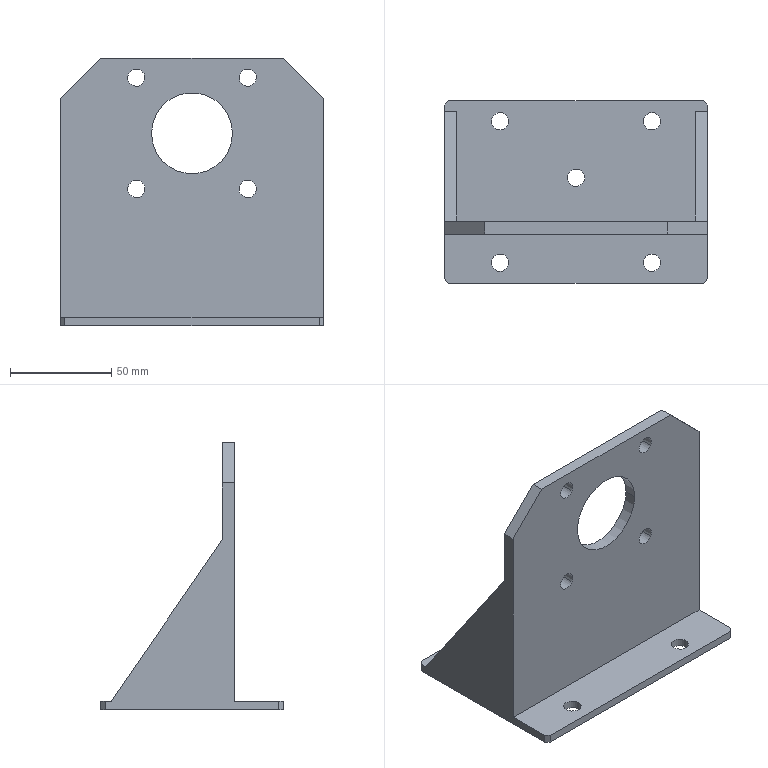Part | STEP file | 20314 | 1 solid | 40 faces | box 130 x 90 x 132 mm | volume 160571 mm3 | cylinder 20 | plane 20 | commonest cylinder face diameters 8.5 x18 40 x2
STEP:
#1=CARTESIAN_POINT('',(23.77,-15.,124.538));
#2=VERTEX_POINT('',#1);
#3=CARTESIAN_POINT('',(23.77,-21.,124.538));
#4=VERTEX_POINT('',#3);
#5=CARTESIAN_POINT('',(23.77,-28.155,124.538));
#6=DIRECTION('',(0.,1.,0.));
#7=VECTOR('',#6,1.);
#8=LINE('',#5,#7);
#9=EDGE_CURVE('',#2,#4,#8,.F.);
#10=ORIENTED_EDGE('',*,*,#9,.F.);
#11=CARTESIAN_POINT('',(31.23,-15.,120.462));
#12=VERTEX_POINT('',#11);
#13=CARTESIAN_POINT('',(27.5,-15.,122.5));
#14=DIRECTION('',(0.,1.,0.));
#15=AXIS2_PLACEMENT_3D('',#13,#14,$);
#16=CIRCLE('',#15,4.25);
#17=EDGE_CURVE('',#12,#2,#16,.F.);
#18=ORIENTED_EDGE('',*,*,#17,.F.);
#19=CARTESIAN_POINT('',(31.23,-21.,120.462));
#20=VERTEX_POINT('',#19);
#21=CARTESIAN_POINT('',(31.23,-28.155,120.462));
#22=DIRECTION('',(0.,1.,0.));
#23=VECTOR('',#22,1.);
#24=LINE('',#21,#23);
#25=EDGE_CURVE('',#12,#20,#24,.F.);
#26=ORIENTED_EDGE('',*,*,#25,.T.);
#27=CARTESIAN_POINT('',(27.5,-21.,122.5));
#28=DIRECTION('',(0.,1.,0.));
#29=AXIS2_PLACEMENT_3D('',#27,#28,$);
#30=CIRCLE('',#29,4.25);
#31=EDGE_CURVE('',#4,#20,#30,.T.);
#32=ORIENTED_EDGE('',*,*,#31,.F.);
#33=EDGE_LOOP('',(#10,#18,#26,#32));
#34=FACE_OUTER_BOUND('',#33,.T.);
#35=CARTESIAN_POINT('',(27.5,-20.9,122.5));
#36=DIRECTION('',(0.,1.,0.));
#37=DIRECTION('',(0.8776,0.,-0.4794));
#38=AXIS2_PLACEMENT_3D('',#35,#36,#37);
#39=CYLINDRICAL_SURFACE('',#38,4.25);
#40=ADVANCED_FACE('',(#34),#39,.F.);
#41=ORIENTED_EDGE('',*,*,#25,.F.);
#42=CARTESIAN_POINT('',(27.5,-15.,122.5));
#43=DIRECTION('',(0.,1.,0.));
#44=AXIS2_PLACEMENT_3D('',#42,#43,$);
#45=CIRCLE('',#44,4.25);
#46=EDGE_CURVE('',#2,#12,#45,.F.);
#47=ORIENTED_EDGE('',*,*,#46,.F.);
#48=ORIENTED_EDGE('',*,*,#9,.T.);
#49=CARTESIAN_POINT('',(27.5,-21.,122.5));
#50=DIRECTION('',(0.,1.,0.));
#51=AXIS2_PLACEMENT_3D('',#49,#50,$);
#52=CIRCLE('',#51,4.25);
#53=EDGE_CURVE('',#20,#4,#52,.T.);
#54=ORIENTED_EDGE('',*,*,#53,.F.);
#55=EDGE_LOOP('',(#41,#47,#48,#54));
#56=FACE_OUTER_BOUND('',#55,.T.);
#57=ADVANCED_FACE('',(#56),#39,.F.);
#58=CARTESIAN_POINT('',(65.,-21.,112.));
#59=VERTEX_POINT('',#58);
#60=CARTESIAN_POINT('',(65.,-15.,112.));
#61=VERTEX_POINT('',#60);
#62=CARTESIAN_POINT('',(65.,-18.,112.));
#63=DIRECTION('',(0.,1.,0.));
#64=VECTOR('',#63,1.);
#65=LINE('',#62,#64);
#66=EDGE_CURVE('',#59,#61,#65,.T.);
#67=ORIENTED_EDGE('',*,*,#66,.F.);
#68=CARTESIAN_POINT('',(65.,-21.,4.));
#69=VERTEX_POINT('',#68);
#70=CARTESIAN_POINT('',(65.,-21.,58.));
#71=DIRECTION('',(0.,0.,1.));
#72=VECTOR('',#71,1.);
#73=LINE('',#70,#72);
#74=EDGE_CURVE('',#69,#59,#73,.T.);
#75=ORIENTED_EDGE('',*,*,#74,.F.);
#76=CARTESIAN_POINT('',(65.,-43.,4.));
#77=VERTEX_POINT('',#76);
#78=CARTESIAN_POINT('',(65.,-32.,4.));
#79=DIRECTION('',(0.,-1.,0.));
#80=VECTOR('',#79,1.);
#81=LINE('',#78,#80);
#82=EDGE_CURVE('',#77,#69,#81,.F.);
#83=ORIENTED_EDGE('',*,*,#82,.F.);
#84=CARTESIAN_POINT('',(65.,-43.,0.));
#85=VERTEX_POINT('',#84);
#86=CARTESIAN_POINT('',(65.,-43.,2.));
#87=DIRECTION('',(0.,0.,1.));
#88=VECTOR('',#87,1.);
#89=LINE('',#86,#88);
#90=EDGE_CURVE('',#85,#77,#89,.T.);
#91=ORIENTED_EDGE('',*,*,#90,.F.);
#92=CARTESIAN_POINT('',(65.,43.,0.));
#93=VERTEX_POINT('',#92);
#94=CARTESIAN_POINT('',(65.,0.,0.));
#95=DIRECTION('',(0.,-1.,0.));
#96=VECTOR('',#95,1.);
#97=LINE('',#94,#96);
#98=EDGE_CURVE('',#85,#93,#97,.F.);
#99=ORIENTED_EDGE('',*,*,#98,.T.);
#100=CARTESIAN_POINT('',(65.,43.,4.));
#101=VERTEX_POINT('',#100);
#102=CARTESIAN_POINT('',(65.,43.,2.));
#103=DIRECTION('',(0.,0.,-1.));
#104=VECTOR('',#103,1.);
#105=LINE('',#102,#104);
#106=EDGE_CURVE('',#93,#101,#105,.F.);
#107=ORIENTED_EDGE('',*,*,#106,.T.);
#108=CARTESIAN_POINT('',(65.,40.,4.));
#109=VERTEX_POINT('',#108);
#110=CARTESIAN_POINT('',(65.,41.5,4.));
#111=DIRECTION('',(0.,-1.,0.));
#112=VECTOR('',#111,1.);
#113=LINE('',#110,#112);
#114=EDGE_CURVE('',#109,#101,#113,.F.);
#115=ORIENTED_EDGE('',*,*,#114,.F.);
#116=CARTESIAN_POINT('',(65.,-15.,84.));
#117=VERTEX_POINT('',#116);
#118=CARTESIAN_POINT('',(65.,12.5,44.));
#119=DIRECTION('',(0.,0.5665,-0.824));
#120=VECTOR('',#119,1.);
#121=LINE('',#118,#120);
#122=EDGE_CURVE('',#117,#109,#121,.T.);
#123=ORIENTED_EDGE('',*,*,#122,.F.);
#124=CARTESIAN_POINT('',(65.,-15.,98.));
#125=DIRECTION('',(0.,0.,1.));
#126=VECTOR('',#125,1.);
#127=LINE('',#124,#126);
#128=EDGE_CURVE('',#117,#61,#127,.T.);
#129=ORIENTED_EDGE('',*,*,#128,.T.);
#130=EDGE_LOOP('',(#67,#75,#83,#91,#99,#107,#115,#123,#129));
#131=FACE_OUTER_BOUND('',#130,.T.);
#132=CARTESIAN_POINT('',(65.,45.,0.));
#133=DIRECTION('',(-1.,0.,0.));
#134=DIRECTION('',(0.,-1.,0.));
#135=AXIS2_PLACEMENT_3D('',#132,#133,#134);
#136=PLANE('',#135);
#137=ADVANCED_FACE('',(#131),#136,.F.);
#138=CARTESIAN_POINT('',(-65.,-21.,4.));
#139=VERTEX_POINT('',#138);
#140=CARTESIAN_POINT('',(-65.,-43.,4.));
#141=VERTEX_POINT('',#140);
#142=CARTESIAN_POINT('',(-65.,-32.,4.));
#143=DIRECTION('',(0.,1.,0.));
#144=VECTOR('',#143,1.);
#145=LINE('',#142,#144);
#146=EDGE_CURVE('',#139,#141,#145,.F.);
#147=ORIENTED_EDGE('',*,*,#146,.T.);
#148=CARTESIAN_POINT('',(-63.,-45.,4.));
#149=VERTEX_POINT('',#148);
#150=CARTESIAN_POINT('',(-64.,-44.,4.));
#151=DIRECTION('',(0.7071,-0.7071,0.));
#152=VECTOR('',#151,1.);
#153=LINE('',#150,#152);
#154=EDGE_CURVE('',#149,#141,#153,.F.);
#155=ORIENTED_EDGE('',*,*,#154,.F.);
#156=CARTESIAN_POINT('',(63.,-45.,4.));
#157=VERTEX_POINT('',#156);
#158=CARTESIAN_POINT('',(0.,-45.,4.));
#159=DIRECTION('',(-1.,0.,0.));
#160=VECTOR('',#159,1.);
#161=LINE('',#158,#160);
#162=EDGE_CURVE('',#149,#157,#161,.F.);
#163=ORIENTED_EDGE('',*,*,#162,.T.);
#164=CARTESIAN_POINT('',(64.,-44.,4.));
#165=DIRECTION('',(-0.7071,-0.7071,0.));
#166=VECTOR('',#165,1.);
#167=LINE('',#164,#166);
#168=EDGE_CURVE('',#77,#157,#167,.T.);
#169=ORIENTED_EDGE('',*,*,#168,.F.);
#170=ORIENTED_EDGE('',*,*,#82,.T.);
#171=CARTESIAN_POINT('',(0.,-21.,4.));
#172=DIRECTION('',(-1.,0.,0.));
#173=VECTOR('',#172,1.);
#174=LINE('',#171,#173);
#175=EDGE_CURVE('',#139,#69,#174,.F.);
#176=ORIENTED_EDGE('',*,*,#175,.F.);
#177=EDGE_LOOP('',(#147,#155,#163,#169,#170,#176));
#178=FACE_OUTER_BOUND('',#177,.T.);
#179=CARTESIAN_POINT('',(41.23,-37.038,4.));
#180=VERTEX_POINT('',#179);
#181=CARTESIAN_POINT('',(33.77,-32.962,4.));
#182=VERTEX_POINT('',#181);
#183=CARTESIAN_POINT('',(37.5,-35.,4.));
#184=DIRECTION('',(0.,0.,1.));
#185=AXIS2_PLACEMENT_3D('',#183,#184,$);
#186=CIRCLE('',#185,4.25);
#187=EDGE_CURVE('',#180,#182,#186,.T.);
#188=ORIENTED_EDGE('',*,*,#187,.F.);
#189=CARTESIAN_POINT('',(37.5,-35.,4.));
#190=DIRECTION('',(0.,0.,1.));
#191=AXIS2_PLACEMENT_3D('',#189,#190,$);
#192=CIRCLE('',#191,4.25);
#193=EDGE_CURVE('',#182,#180,#192,.T.);
#194=ORIENTED_EDGE('',*,*,#193,.F.);
#195=EDGE_LOOP('',(#188,#194));
#196=FACE_BOUND('',#195,.T.);
#197=CARTESIAN_POINT('',(-33.77,-37.038,4.));
#198=VERTEX_POINT('',#197);
#199=CARTESIAN_POINT('',(-41.23,-32.962,4.));
#200=VERTEX_POINT('',#199);
#201=CARTESIAN_POINT('',(-37.5,-35.,4.));
#202=DIRECTION('',(0.,0.,1.));
#203=AXIS2_PLACEMENT_3D('',#201,#202,$);
#204=CIRCLE('',#203,4.25);
#205=EDGE_CURVE('',#198,#200,#204,.T.);
#206=ORIENTED_EDGE('',*,*,#205,.F.);
#207=CARTESIAN_POINT('',(-37.5,-35.,4.));
#208=DIRECTION('',(0.,0.,1.));
#209=AXIS2_PLACEMENT_3D('',#207,#208,$);
#210=CIRCLE('',#209,4.25);
#211=EDGE_CURVE('',#200,#198,#210,.T.);
#212=ORIENTED_EDGE('',*,*,#211,.F.);
#213=EDGE_LOOP('',(#206,#212));
#214=FACE_BOUND('',#213,.T.);
#215=CARTESIAN_POINT('',(0.,0.,4.));
#216=DIRECTION('',(0.,0.,1.));
#217=DIRECTION('',(1.,0.,0.));
#218=AXIS2_PLACEMENT_3D('',#215,#216,#217);
#219=PLANE('',#218);
#220=ADVANCED_FACE('',(#178,#196,#214),#219,.T.);
#221=ORIENTED_EDGE('',*,*,#106,.F.);
#222=CARTESIAN_POINT('',(63.,45.,0.));
#223=VERTEX_POINT('',#222);
#224=CARTESIAN_POINT('',(64.,44.,0.));
#225=DIRECTION('',(0.7071,-0.7071,0.));
#226=VECTOR('',#225,1.);
#227=LINE('',#224,#226);
#228=EDGE_CURVE('',#93,#223,#227,.F.);
#229=ORIENTED_EDGE('',*,*,#228,.T.);
#230=CARTESIAN_POINT('',(63.,45.,4.));
#231=VERTEX_POINT('',#230);
#232=CARTESIAN_POINT('',(63.,45.,2.));
#233=DIRECTION('',(0.,0.,-1.));
#234=VECTOR('',#233,1.);
#235=LINE('',#232,#234);
#236=EDGE_CURVE('',#223,#231,#235,.F.);
#237=ORIENTED_EDGE('',*,*,#236,.T.);
#238=CARTESIAN_POINT('',(64.,44.,4.));
#239=DIRECTION('',(0.7071,-0.7071,0.));
#240=VECTOR('',#239,1.);
#241=LINE('',#238,#240);
#242=EDGE_CURVE('',#231,#101,#241,.T.);
#243=ORIENTED_EDGE('',*,*,#242,.T.);
#244=EDGE_LOOP('',(#221,#229,#237,#243));
#245=FACE_OUTER_BOUND('',#244,.T.);
#246=CARTESIAN_POINT('',(63.,45.,4.8));
#247=DIRECTION('',(-0.7071,-0.7071,0.));
#248=DIRECTION('',(0.,0.,-1.));
#249=AXIS2_PLACEMENT_3D('',#246,#247,#248);
#250=PLANE('',#249);
#251=ADVANCED_FACE('',(#245),#250,.F.);
#252=CARTESIAN_POINT('',(-65.,-43.,0.));
#253=VERTEX_POINT('',#252);
#254=CARTESIAN_POINT('',(-63.,-45.,0.));
#255=VERTEX_POINT('',#254);
#256=CARTESIAN_POINT('',(-64.,-44.,0.));
#257=DIRECTION('',(0.7071,-0.7071,0.));
#258=VECTOR('',#257,1.);
#259=LINE('',#256,#258);
#260=EDGE_CURVE('',#253,#255,#259,.T.);
#261=ORIENTED_EDGE('',*,*,#260,.F.);
#262=CARTESIAN_POINT('',(-65.,43.,0.));
#263=VERTEX_POINT('',#262);
#264=CARTESIAN_POINT('',(-65.,0.,0.));
#265=DIRECTION('',(0.,1.,0.));
#266=VECTOR('',#265,1.);
#267=LINE('',#264,#266);
#268=EDGE_CURVE('',#263,#253,#267,.F.);
#269=ORIENTED_EDGE('',*,*,#268,.F.);
#270=CARTESIAN_POINT('',(-63.,45.,0.));
#271=VERTEX_POINT('',#270);
#272=CARTESIAN_POINT('',(-64.,44.,0.));
#273=DIRECTION('',(0.7071,0.7071,0.));
#274=VECTOR('',#273,1.);
#275=LINE('',#272,#274);
#276=EDGE_CURVE('',#271,#263,#275,.F.);
#277=ORIENTED_EDGE('',*,*,#276,.F.);
#278=CARTESIAN_POINT('',(0.,45.,0.));
#279=DIRECTION('',(1.,0.,0.));
#280=VECTOR('',#279,1.);
#281=LINE('',#278,#280);
#282=EDGE_CURVE('',#223,#271,#281,.F.);
#283=ORIENTED_EDGE('',*,*,#282,.F.);
#284=ORIENTED_EDGE('',*,*,#228,.F.);
#285=ORIENTED_EDGE('',*,*,#98,.F.);
#286=CARTESIAN_POINT('',(63.,-45.,0.));
#287=VERTEX_POINT('',#286);
#288=CARTESIAN_POINT('',(64.,-44.,0.));
#289=DIRECTION('',(-0.7071,-0.7071,0.));
#290=VECTOR('',#289,1.);
#291=LINE('',#288,#290);
#292=EDGE_CURVE('',#287,#85,#291,.F.);
#293=ORIENTED_EDGE('',*,*,#292,.F.);
#294=CARTESIAN_POINT('',(0.,-45.,0.));
#295=DIRECTION('',(-1.,0.,0.));
#296=VECTOR('',#295,1.);
#297=LINE('',#294,#296);
#298=EDGE_CURVE('',#255,#287,#297,.F.);
#299=ORIENTED_EDGE('',*,*,#298,.F.);
#300=EDGE_LOOP('',(#261,#269,#277,#283,#284,#285,#293,#299));
#301=FACE_OUTER_BOUND('',#300,.T.);
#302=CARTESIAN_POINT('',(33.77,-32.962,0.));
#303=VERTEX_POINT('',#302);
#304=CARTESIAN_POINT('',(41.23,-37.038,0.));
#305=VERTEX_POINT('',#304);
#306=CARTESIAN_POINT('',(37.5,-35.,0.));
#307=DIRECTION('',(0.,0.,1.));
#308=AXIS2_PLACEMENT_3D('',#306,#307,$);
#309=CIRCLE('',#308,4.25);
#310=EDGE_CURVE('',#303,#305,#309,.T.);
#311=ORIENTED_EDGE('',*,*,#310,.T.);
#312=CARTESIAN_POINT('',(37.5,-35.,0.));
#313=DIRECTION('',(0.,0.,1.));
#314=AXIS2_PLACEMENT_3D('',#312,#313,$);
#315=CIRCLE('',#314,4.25);
#316=EDGE_CURVE('',#305,#303,#315,.T.);
#317=ORIENTED_EDGE('',*,*,#316,.T.);
#318=EDGE_LOOP('',(#311,#317));
#319=FACE_BOUND('',#318,.T.);
#320=CARTESIAN_POINT('',(41.23,32.962,0.));
#321=VERTEX_POINT('',#320);
#322=CARTESIAN_POINT('',(33.77,37.038,0.));
#323=VERTEX_POINT('',#322);
#324=CARTESIAN_POINT('',(37.5,35.,0.));
#325=DIRECTION('',(0.,0.,1.));
#326=AXIS2_PLACEMENT_3D('',#324,#325,$);
#327=CIRCLE('',#326,4.25);
#328=EDGE_CURVE('',#321,#323,#327,.T.);
#329=ORIENTED_EDGE('',*,*,#328,.T.);
#330=CARTESIAN_POINT('',(37.5,35.,0.));
#331=DIRECTION('',(0.,0.,1.));
#332=AXIS2_PLACEMENT_3D('',#330,#331,$);
#333=CIRCLE('',#332,4.25);
#334=EDGE_CURVE('',#323,#321,#333,.T.);
#335=ORIENTED_EDGE('',*,*,#334,.T.);
#336=EDGE_LOOP('',(#329,#335));
#337=FACE_BOUND('',#336,.T.);
#338=CARTESIAN_POINT('',(-41.23,-32.962,0.));
#339=VERTEX_POINT('',#338);
#340=CARTESIAN_POINT('',(-33.77,-37.038,0.));
#341=VERTEX_POINT('',#340);
#342=CARTESIAN_POINT('',(-37.5,-35.,0.));
#343=DIRECTION('',(0.,0.,1.));
#344=AXIS2_PLACEMENT_3D('',#342,#343,$);
#345=CIRCLE('',#344,4.25);
#346=EDGE_CURVE('',#339,#341,#345,.T.);
#347=ORIENTED_EDGE('',*,*,#346,.T.);
#348=CARTESIAN_POINT('',(-37.5,-35.,0.));
#349=DIRECTION('',(0.,0.,1.));
#350=AXIS2_PLACEMENT_3D('',#348,#349,$);
#351=CIRCLE('',#350,4.25);
#352=EDGE_CURVE('',#341,#339,#351,.T.);
#353=ORIENTED_EDGE('',*,*,#352,.T.);
#354=EDGE_LOOP('',(#347,#353));
#355=FACE_BOUND('',#354,.T.);
#356=CARTESIAN_POINT('',(-41.23,37.038,0.));
#357=VERTEX_POINT('',#356);
#358=CARTESIAN_POINT('',(-33.77,32.962,0.));
#359=VERTEX_POINT('',#358);
#360=CARTESIAN_POINT('',(-37.5,35.,0.));
#361=DIRECTION('',(0.,0.,1.));
#362=AXIS2_PLACEMENT_3D('',#360,#361,$);
#363=CIRCLE('',#362,4.25);
#364=EDGE_CURVE('',#357,#359,#363,.T.);
#365=ORIENTED_EDGE('',*,*,#364,.T.);
#366=CARTESIAN_POINT('',(-37.5,35.,0.));
#367=DIRECTION('',(0.,0.,1.));
#368=AXIS2_PLACEMENT_3D('',#366,#367,$);
#369=CIRCLE('',#368,4.25);
#370=EDGE_CURVE('',#359,#357,#369,.T.);
#371=ORIENTED_EDGE('',*,*,#370,.T.);
#372=EDGE_LOOP('',(#365,#371));
#373=FACE_BOUND('',#372,.T.);
#374=CARTESIAN_POINT('',(-3.73,9.038,0.));
#375=VERTEX_POINT('',#374);
#376=CARTESIAN_POINT('',(3.73,4.962,0.));
#377=VERTEX_POINT('',#376);
#378=CARTESIAN_POINT('',(0.,7.,0.));
#379=DIRECTION('',(0.,0.,1.));
#380=AXIS2_PLACEMENT_3D('',#378,#379,$);
#381=CIRCLE('',#380,4.25);
#382=EDGE_CURVE('',#375,#377,#381,.T.);
#383=ORIENTED_EDGE('',*,*,#382,.T.);
#384=CARTESIAN_POINT('',(0.,7.,0.));
#385=DIRECTION('',(0.,0.,1.));
#386=AXIS2_PLACEMENT_3D('',#384,#385,$);
#387=CIRCLE('',#386,4.25);
#388=EDGE_CURVE('',#377,#375,#387,.T.);
#389=ORIENTED_EDGE('',*,*,#388,.T.);
#390=EDGE_LOOP('',(#383,#389));
#391=FACE_BOUND('',#390,.T.);
#392=CARTESIAN_POINT('',(0.,0.,0.));
#393=DIRECTION('',(0.,0.,1.));
#394=DIRECTION('',(1.,0.,0.));
#395=AXIS2_PLACEMENT_3D('',#392,#393,#394);
#396=PLANE('',#395);
#397=ADVANCED_FACE('',(#301,#319,#337,#355,#373,#391),#396,.F.);
#398=CARTESIAN_POINT('',(-63.,-45.,2.));
#399=DIRECTION('',(0.,0.,-1.));
#400=VECTOR('',#399,1.);
#401=LINE('',#398,#400);
#402=EDGE_CURVE('',#255,#149,#401,.F.);
#403=ORIENTED_EDGE('',*,*,#402,.F.);
#404=ORIENTED_EDGE('',*,*,#298,.T.);
#405=CARTESIAN_POINT('',(63.,-45.,2.));
#406=DIRECTION('',(0.,0.,1.));
#407=VECTOR('',#406,1.);
#408=LINE('',#405,#407);
#409=EDGE_CURVE('',#287,#157,#408,.T.);
#410=ORIENTED_EDGE('',*,*,#409,.T.);
#411=ORIENTED_EDGE('',*,*,#162,.F.);
#412=EDGE_LOOP('',(#403,#404,#410,#411));
#413=FACE_OUTER_BOUND('',#412,.T.);
#414=CARTESIAN_POINT('',(65.,-45.,0.));
#415=DIRECTION('',(0.,1.,0.));
#416=DIRECTION('',(-1.,0.,0.));
#417=AXIS2_PLACEMENT_3D('',#414,#415,#416);
#418=PLANE('',#417);
#419=ADVANCED_FACE('',(#413),#418,.F.);
#420=CARTESIAN_POINT('',(-63.,45.,4.));
#421=VERTEX_POINT('',#420);
#422=CARTESIAN_POINT('',(-63.,45.,2.));
#423=DIRECTION('',(0.,0.,1.));
#424=VECTOR('',#423,1.);
#425=LINE('',#422,#424);
#426=EDGE_CURVE('',#271,#421,#425,.T.);
#427=ORIENTED_EDGE('',*,*,#426,.T.);
#428=CARTESIAN_POINT('',(0.,45.,4.));
#429=DIRECTION('',(1.,0.,0.));
#430=VECTOR('',#429,1.);
#431=LINE('',#428,#430);
#432=EDGE_CURVE('',#231,#421,#431,.F.);
#433=ORIENTED_EDGE('',*,*,#432,.F.);
#434=ORIENTED_EDGE('',*,*,#236,.F.);
#435=ORIENTED_EDGE('',*,*,#282,.T.);
#436=EDGE_LOOP('',(#427,#433,#434,#435));
#437=FACE_OUTER_BOUND('',#436,.T.);
#438=CARTESIAN_POINT('',(-65.,45.,0.));
#439=DIRECTION('',(0.,-1.,0.));
#440=DIRECTION('',(1.,0.,0.));
#441=AXIS2_PLACEMENT_3D('',#438,#439,#440);
#442=PLANE('',#441);
#443=ADVANCED_FACE('',(#437),#442,.F.);
#444=CARTESIAN_POINT('',(41.23,32.962,4.));
#445=VERTEX_POINT('',#444);
#446=CARTESIAN_POINT('',(41.23,32.962,-0.845));
#447=DIRECTION('',(0.,0.,-1.));
#448=VECTOR('',#447,1.);
#449=LINE('',#446,#448);
#450=EDGE_CURVE('',#321,#445,#449,.F.);
#451=ORIENTED_EDGE('',*,*,#450,.F.);
#452=ORIENTED_EDGE('',*,*,#334,.F.);
#453=CARTESIAN_POINT('',(33.77,37.038,4.));
#454=VERTEX_POINT('',#453);
#455=CARTESIAN_POINT('',(33.77,37.038,-0.845));
#456=DIRECTION('',(0.,0.,-1.));
#457=VECTOR('',#456,1.);
#458=LINE('',#455,#457);
#459=EDGE_CURVE('',#323,#454,#458,.F.);
#460=ORIENTED_EDGE('',*,*,#459,.T.);
#461=CARTESIAN_POINT('',(37.5,35.,4.));
#462=DIRECTION('',(0.,0.,-1.));
#463=AXIS2_PLACEMENT_3D('',#461,#462,$);
#464=CIRCLE('',#463,4.25);
#465=EDGE_CURVE('',#454,#445,#464,.F.);
#466=ORIENTED_EDGE('',*,*,#465,.T.);
#467=EDGE_LOOP('',(#451,#452,#460,#466));
#468=FACE_OUTER_BOUND('',#467,.T.);
#469=CARTESIAN_POINT('',(37.5,35.,3.9));
#470=DIRECTION('',(0.,0.,-1.));
#471=DIRECTION('',(0.8776,-0.4794,0.));
#472=AXIS2_PLACEMENT_3D('',#469,#470,#471);
#473=CYLINDRICAL_SURFACE('',#472,4.25);
#474=ADVANCED_FACE('',(#468),#473,.F.);
#475=ORIENTED_EDGE('',*,*,#459,.F.);
#476=ORIENTED_EDGE('',*,*,#328,.F.);
#477=ORIENTED_EDGE('',*,*,#450,.T.);
#478=CARTESIAN_POINT('',(37.5,35.,4.));
#479=DIRECTION('',(0.,0.,-1.));
#480=AXIS2_PLACEMENT_3D('',#478,#479,$);
#481=CIRCLE('',#480,4.25);
#482=EDGE_CURVE('',#445,#454,#481,.F.);
#483=ORIENTED_EDGE('',*,*,#482,.T.);
#484=EDGE_LOOP('',(#475,#476,#477,#483));
#485=FACE_OUTER_BOUND('',#484,.T.);
#486=ADVANCED_FACE('',(#485),#473,.F.);
#487=CARTESIAN_POINT('',(-41.23,37.038,4.));
#488=VERTEX_POINT('',#487);
#489=CARTESIAN_POINT('',(-41.23,37.038,-0.845));
#490=DIRECTION('',(0.,0.,-1.));
#491=VECTOR('',#490,1.);
#492=LINE('',#489,#491);
#493=EDGE_CURVE('',#357,#488,#492,.F.);
#494=ORIENTED_EDGE('',*,*,#493,.F.);
#495=ORIENTED_EDGE('',*,*,#370,.F.);
#496=CARTESIAN_POINT('',(-33.77,32.962,4.));
#497=VERTEX_POINT('',#496);
#498=CARTESIAN_POINT('',(-33.77,32.962,-0.845));
#499=DIRECTION('',(0.,0.,-1.));
#500=VECTOR('',#499,1.);
#501=LINE('',#498,#500);
#502=EDGE_CURVE('',#359,#497,#501,.F.);
#503=ORIENTED_EDGE('',*,*,#502,.T.);
#504=CARTESIAN_POINT('',(-37.5,35.,4.));
#505=DIRECTION('',(0.,0.,-1.));
#506=AXIS2_PLACEMENT_3D('',#504,#505,$);
#507=CIRCLE('',#506,4.25);
#508=EDGE_CURVE('',#497,#488,#507,.F.);
#509=ORIENTED_EDGE('',*,*,#508,.T.);
#510=EDGE_LOOP('',(#494,#495,#503,#509));
#511=FACE_OUTER_BOUND('',#510,.T.);
#512=CARTESIAN_POINT('',(-37.5,35.,3.9));
#513=DIRECTION('',(0.,0.,-1.));
#514=DIRECTION('',(0.8776,-0.4794,0.));
#515=AXIS2_PLACEMENT_3D('',#512,#513,#514);
#516=CYLINDRICAL_SURFACE('',#515,4.25);
#517=ADVANCED_FACE('',(#511),#516,.F.);
#518=ORIENTED_EDGE('',*,*,#502,.F.);
#519=ORIENTED_EDGE('',*,*,#364,.F.);
#520=ORIENTED_EDGE('',*,*,#493,.T.);
#521=CARTESIAN_POINT('',(-37.5,35.,4.));
#522=DIRECTION('',(0.,0.,-1.));
#523=AXIS2_PLACEMENT_3D('',#521,#522,$);
#524=CIRCLE('',#523,4.25);
#525=EDGE_CURVE('',#488,#497,#524,.F.);
#526=ORIENTED_EDGE('',*,*,#525,.T.);
#527=EDGE_LOOP('',(#518,#519,#520,#526));
#528=FACE_OUTER_BOUND('',#527,.T.);
#529=ADVANCED_FACE('',(#528),#516,.F.);
#530=CARTESIAN_POINT('',(-3.73,9.038,4.));
#531=VERTEX_POINT('',#530);
#532=CARTESIAN_POINT('',(-3.73,9.038,-0.845));
#533=DIRECTION('',(0.,0.,-1.));
#534=VECTOR('',#533,1.);
#535=LINE('',#532,#534);
#536=EDGE_CURVE('',#375,#531,#535,.F.);
#537=ORIENTED_EDGE('',*,*,#536,.F.);
#538=ORIENTED_EDGE('',*,*,#388,.F.);
#539=CARTESIAN_POINT('',(3.73,4.962,4.));
#540=VERTEX_POINT('',#539);
#541=CARTESIAN_POINT('',(3.73,4.962,-0.845));
#542=DIRECTION('',(0.,0.,-1.));
#543=VECTOR('',#542,1.);
#544=LINE('',#541,#543);
#545=EDGE_CURVE('',#377,#540,#544,.F.);
#546=ORIENTED_EDGE('',*,*,#545,.T.);
#547=CARTESIAN_POINT('',(0.,7.,4.));
#548=DIRECTION('',(0.,0.,-1.));
#549=AXIS2_PLACEMENT_3D('',#547,#548,$);
#550=CIRCLE('',#549,4.25);
#551=EDGE_CURVE('',#540,#531,#550,.F.);
#552=ORIENTED_EDGE('',*,*,#551,.T.);
#553=EDGE_LOOP('',(#537,#538,#546,#552));
#554=FACE_OUTER_BOUND('',#553,.T.);
#555=CARTESIAN_POINT('',(0.,7.,3.9));
#556=DIRECTION('',(0.,0.,-1.));
#557=DIRECTION('',(0.8776,-0.4794,0.));
#558=AXIS2_PLACEMENT_3D('',#555,#556,#557);
#559=CYLINDRICAL_SURFACE('',#558,4.25);
#560=ADVANCED_FACE('',(#554),#559,.F.);
#561=ORIENTED_EDGE('',*,*,#545,.F.);
#562=ORIENTED_EDGE('',*,*,#382,.F.);
#563=ORIENTED_EDGE('',*,*,#536,.T.);
#564=CARTESIAN_POINT('',(0.,7.,4.));
#565=DIRECTION('',(0.,0.,-1.));
#566=AXIS2_PLACEMENT_3D('',#564,#565,$);
#567=CIRCLE('',#566,4.25);
#568=EDGE_CURVE('',#531,#540,#567,.F.);
#569=ORIENTED_EDGE('',*,*,#568,.T.);
#570=EDGE_LOOP('',(#561,#562,#563,#569));
#571=FACE_OUTER_BOUND('',#570,.T.);
#572=ADVANCED_FACE('',(#571),#559,.F.);
#573=CARTESIAN_POINT('',(-59.,-15.,84.));
#574=VERTEX_POINT('',#573);
#575=CARTESIAN_POINT('',(-65.,-15.,84.));
#576=VERTEX_POINT('',#575);
#577=CARTESIAN_POINT('',(-62.,-15.,84.));
#578=DIRECTION('',(-1.,0.,0.));
#579=VECTOR('',#578,1.);
#580=LINE('',#577,#579);
#581=EDGE_CURVE('',#574,#576,#580,.T.);
#582=ORIENTED_EDGE('',*,*,#581,.F.);
#583=CARTESIAN_POINT('',(-59.,40.,4.));
#584=VERTEX_POINT('',#583);
#585=CARTESIAN_POINT('',(-59.,12.5,44.));
#586=DIRECTION('',(0.,0.5665,-0.824));
#587=VECTOR('',#586,1.);
#588=LINE('',#585,#587);
#589=EDGE_CURVE('',#574,#584,#588,.T.);
#590=ORIENTED_EDGE('',*,*,#589,.T.);
#591=CARTESIAN_POINT('',(-65.,40.,4.));
#592=VERTEX_POINT('',#591);
#593=CARTESIAN_POINT('',(-62.,40.,4.));
#594=DIRECTION('',(-1.,0.,0.));
#595=VECTOR('',#594,1.);
#596=LINE('',#593,#595);
#597=EDGE_CURVE('',#584,#592,#596,.T.);
#598=ORIENTED_EDGE('',*,*,#597,.T.);
#599=CARTESIAN_POINT('',(-65.,12.5,44.));
#600=DIRECTION('',(0.,0.5665,-0.824));
#601=VECTOR('',#600,1.);
#602=LINE('',#599,#601);
#603=EDGE_CURVE('',#576,#592,#602,.T.);
#604=ORIENTED_EDGE('',*,*,#603,.F.);
#605=EDGE_LOOP('',(#582,#590,#598,#604));
#606=FACE_OUTER_BOUND('',#605,.T.);
#607=CARTESIAN_POINT('',(0.,-15.,84.));
#608=DIRECTION('',(0.,0.824,0.5665));
#609=DIRECTION('',(0.,0.5665,-0.824));
#610=AXIS2_PLACEMENT_3D('',#607,#608,#609);
#611=PLANE('',#610);
#612=ADVANCED_FACE('',(#606),#611,.T.);
#613=CARTESIAN_POINT('',(59.,40.,4.));
#614=VERTEX_POINT('',#613);
#615=CARTESIAN_POINT('',(59.,-15.,4.));
#616=VERTEX_POINT('',#615);
#617=CARTESIAN_POINT('',(59.,12.5,4.));
#618=DIRECTION('',(0.,-1.,0.));
#619=VECTOR('',#618,1.);
#620=LINE('',#617,#619);
#621=EDGE_CURVE('',#614,#616,#620,.T.);
#622=ORIENTED_EDGE('',*,*,#621,.T.);
#623=CARTESIAN_POINT('',(59.,-15.,84.));
#624=VERTEX_POINT('',#623);
#625=CARTESIAN_POINT('',(59.,-15.,44.));
#626=DIRECTION('',(0.,0.,-1.));
#627=VECTOR('',#626,1.);
#628=LINE('',#625,#627);
#629=EDGE_CURVE('',#624,#616,#628,.T.);
#630=ORIENTED_EDGE('',*,*,#629,.F.);
#631=CARTESIAN_POINT('',(59.,12.5,44.));
#632=DIRECTION('',(0.,0.5665,-0.824));
#633=VECTOR('',#632,1.);
#634=LINE('',#631,#633);
#635=EDGE_CURVE('',#624,#614,#634,.T.);
#636=ORIENTED_EDGE('',*,*,#635,.T.);
#637=EDGE_LOOP('',(#622,#630,#636));
#638=FACE_OUTER_BOUND('',#637,.T.);
#639=CARTESIAN_POINT('',(59.,0.,56.));
#640=DIRECTION('',(-1.,0.,0.));
#641=DIRECTION('',(0.,-1.,0.));
#642=AXIS2_PLACEMENT_3D('',#639,#640,#641);
#643=PLANE('',#642);
#644=ADVANCED_FACE('',(#638),#643,.T.);
#645=ORIENTED_EDGE('',*,*,#589,.F.);
#646=CARTESIAN_POINT('',(-59.,-15.,4.));
#647=VERTEX_POINT('',#646);
#648=CARTESIAN_POINT('',(-59.,-15.,44.));
#649=DIRECTION('',(0.,0.,-1.));
#650=VECTOR('',#649,1.);
#651=LINE('',#648,#650);
#652=EDGE_CURVE('',#574,#647,#651,.T.);
#653=ORIENTED_EDGE('',*,*,#652,.T.);
#654=CARTESIAN_POINT('',(-59.,12.5,4.));
#655=DIRECTION('',(0.,-1.,0.));
#656=VECTOR('',#655,1.);
#657=LINE('',#654,#656);
#658=EDGE_CURVE('',#584,#647,#657,.T.);
#659=ORIENTED_EDGE('',*,*,#658,.F.);
#660=EDGE_LOOP('',(#645,#653,#659));
#661=FACE_OUTER_BOUND('',#660,.T.);
#662=CARTESIAN_POINT('',(-59.,0.,56.));
#663=DIRECTION('',(1.,0.,0.));
#664=DIRECTION('',(0.,1.,0.));
#665=AXIS2_PLACEMENT_3D('',#662,#663,#664);
#666=PLANE('',#665);
#667=ADVANCED_FACE('',(#661),#666,.T.);
#668=ORIENTED_EDGE('',*,*,#426,.F.);
#669=ORIENTED_EDGE('',*,*,#276,.T.);
#670=CARTESIAN_POINT('',(-65.,43.,4.));
#671=VERTEX_POINT('',#670);
#672=CARTESIAN_POINT('',(-65.,43.,2.));
#673=DIRECTION('',(0.,0.,1.));
#674=VECTOR('',#673,1.);
#675=LINE('',#672,#674);
#676=EDGE_CURVE('',#263,#671,#675,.T.);
#677=ORIENTED_EDGE('',*,*,#676,.T.);
#678=CARTESIAN_POINT('',(-64.,44.,4.));
#679=DIRECTION('',(-0.7071,-0.7071,0.));
#680=VECTOR('',#679,1.);
#681=LINE('',#678,#680);
#682=EDGE_CURVE('',#671,#421,#681,.F.);
#683=ORIENTED_EDGE('',*,*,#682,.T.);
#684=EDGE_LOOP('',(#668,#669,#677,#683));
#685=FACE_OUTER_BOUND('',#684,.T.);
#686=CARTESIAN_POINT('',(-63.,45.,-0.8));
#687=DIRECTION('',(0.7071,-0.7071,0.));
#688=DIRECTION('',(0.,0.,1.));
#689=AXIS2_PLACEMENT_3D('',#686,#687,#688);
#690=PLANE('',#689);
#691=ADVANCED_FACE('',(#685),#690,.F.);
#692=CARTESIAN_POINT('',(-33.77,-37.038,-0.845));
#693=DIRECTION('',(0.,0.,-1.));
#694=VECTOR('',#693,1.);
#695=LINE('',#692,#694);
#696=EDGE_CURVE('',#341,#198,#695,.F.);
#697=ORIENTED_EDGE('',*,*,#696,.F.);
#698=ORIENTED_EDGE('',*,*,#346,.F.);
#699=CARTESIAN_POINT('',(-41.23,-32.962,-0.845));
#700=DIRECTION('',(0.,0.,-1.));
#701=VECTOR('',#700,1.);
#702=LINE('',#699,#701);
#703=EDGE_CURVE('',#339,#200,#702,.F.);
#704=ORIENTED_EDGE('',*,*,#703,.T.);
#705=ORIENTED_EDGE('',*,*,#211,.T.);
#706=EDGE_LOOP('',(#697,#698,#704,#705));
#707=FACE_OUTER_BOUND('',#706,.T.);
#708=CARTESIAN_POINT('',(-37.5,-35.,3.9));
#709=DIRECTION('',(0.,0.,-1.));
#710=DIRECTION('',(0.8776,-0.4794,0.));
#711=AXIS2_PLACEMENT_3D('',#708,#709,#710);
#712=CYLINDRICAL_SURFACE('',#711,4.25);
#713=ADVANCED_FACE('',(#707),#712,.F.);
#714=ORIENTED_EDGE('',*,*,#703,.F.);
#715=ORIENTED_EDGE('',*,*,#352,.F.);
#716=ORIENTED_EDGE('',*,*,#696,.T.);
#717=ORIENTED_EDGE('',*,*,#205,.T.);
#718=EDGE_LOOP('',(#714,#715,#716,#717));
#719=FACE_OUTER_BOUND('',#718,.T.);
#720=ADVANCED_FACE('',(#719),#712,.F.);
#721=CARTESIAN_POINT('',(41.23,-37.038,-0.845));
#722=DIRECTION('',(0.,0.,-1.));
#723=VECTOR('',#722,1.);
#724=LINE('',#721,#723);
#725=EDGE_CURVE('',#305,#180,#724,.F.);
#726=ORIENTED_EDGE('',*,*,#725,.F.);
#727=ORIENTED_EDGE('',*,*,#310,.F.);
#728=CARTESIAN_POINT('',(33.77,-32.962,-0.845));
#729=DIRECTION('',(0.,0.,-1.));
#730=VECTOR('',#729,1.);
#731=LINE('',#728,#730);
#732=EDGE_CURVE('',#303,#182,#731,.F.);
#733=ORIENTED_EDGE('',*,*,#732,.T.);
#734=ORIENTED_EDGE('',*,*,#193,.T.);
#735=EDGE_LOOP('',(#726,#727,#733,#734));
#736=FACE_OUTER_BOUND('',#735,.T.);
#737=CARTESIAN_POINT('',(37.5,-35.,3.9));
#738=DIRECTION('',(0.,0.,-1.));
#739=DIRECTION('',(0.8776,-0.4794,0.));
#740=AXIS2_PLACEMENT_3D('',#737,#738,#739);
#741=CYLINDRICAL_SURFACE('',#740,4.25);
#742=ADVANCED_FACE('',(#736),#741,.F.);
#743=ORIENTED_EDGE('',*,*,#732,.F.);
#744=ORIENTED_EDGE('',*,*,#316,.F.);
#745=ORIENTED_EDGE('',*,*,#725,.T.);
#746=ORIENTED_EDGE('',*,*,#187,.T.);
#747=EDGE_LOOP('',(#743,#744,#745,#746));
#748=FACE_OUTER_BOUND('',#747,.T.);
#749=ADVANCED_FACE('',(#748),#741,.F.);
#750=CARTESIAN_POINT('',(-65.,-43.,2.));
#751=DIRECTION('',(0.,0.,-1.));
#752=VECTOR('',#751,1.);
#753=LINE('',#750,#752);
#754=EDGE_CURVE('',#253,#141,#753,.F.);
#755=ORIENTED_EDGE('',*,*,#754,.F.);
#756=ORIENTED_EDGE('',*,*,#260,.T.);
#757=ORIENTED_EDGE('',*,*,#402,.T.);
#758=ORIENTED_EDGE('',*,*,#154,.T.);
#759=EDGE_LOOP('',(#755,#756,#757,#758));
#760=FACE_OUTER_BOUND('',#759,.T.);
#761=CARTESIAN_POINT('',(-63.,-45.,4.8));
#762=DIRECTION('',(0.7071,0.7071,0.));
#763=DIRECTION('',(0.,0.,-1.));
#764=AXIS2_PLACEMENT_3D('',#761,#762,#763);
#765=PLANE('',#764);
#766=ADVANCED_FACE('',(#760),#765,.F.);
#767=ORIENTED_EDGE('',*,*,#409,.F.);
#768=ORIENTED_EDGE('',*,*,#292,.T.);
#769=ORIENTED_EDGE('',*,*,#90,.T.);
#770=ORIENTED_EDGE('',*,*,#168,.T.);
#771=EDGE_LOOP('',(#767,#768,#769,#770));
#772=FACE_OUTER_BOUND('',#771,.T.);
#773=CARTESIAN_POINT('',(63.,-45.,-0.8));
#774=DIRECTION('',(-0.7071,0.7071,0.));
#775=DIRECTION('',(0.,0.,1.));
#776=AXIS2_PLACEMENT_3D('',#773,#774,#775);
#777=PLANE('',#776);
#778=ADVANCED_FACE('',(#772),#777,.F.);
#779=ORIENTED_EDGE('',*,*,#114,.T.);
#780=ORIENTED_EDGE('',*,*,#242,.F.);
#781=ORIENTED_EDGE('',*,*,#432,.T.);
#782=ORIENTED_EDGE('',*,*,#682,.F.);
#783=CARTESIAN_POINT('',(-65.,41.5,4.));
#784=DIRECTION('',(0.,1.,0.));
#785=VECTOR('',#784,1.);
#786=LINE('',#783,#785);
#787=EDGE_CURVE('',#671,#592,#786,.F.);
#788=ORIENTED_EDGE('',*,*,#787,.T.);
#789=ORIENTED_EDGE('',*,*,#597,.F.);
#790=ORIENTED_EDGE('',*,*,#658,.T.);
#791=CARTESIAN_POINT('',(0.,-15.,4.));
#792=DIRECTION('',(1.,0.,0.));
#793=VECTOR('',#792,1.);
#794=LINE('',#791,#793);
#795=EDGE_CURVE('',#616,#647,#794,.F.);
#796=ORIENTED_EDGE('',*,*,#795,.F.);
#797=ORIENTED_EDGE('',*,*,#621,.F.);
#798=CARTESIAN_POINT('',(62.,40.,4.));
#799=DIRECTION('',(-1.,0.,0.));
#800=VECTOR('',#799,1.);
#801=LINE('',#798,#800);
#802=EDGE_CURVE('',#109,#614,#801,.T.);
#803=ORIENTED_EDGE('',*,*,#802,.F.);
#804=EDGE_LOOP('',(#779,#780,#781,#782,#788,#789,#790,#796,#797,#803));
#805=FACE_OUTER_BOUND('',#804,.T.);
#806=ORIENTED_EDGE('',*,*,#465,.F.);
#807=ORIENTED_EDGE('',*,*,#482,.F.);
#808=EDGE_LOOP('',(#806,#807));
#809=FACE_BOUND('',#808,.T.);
#810=ORIENTED_EDGE('',*,*,#508,.F.);
#811=ORIENTED_EDGE('',*,*,#525,.F.);
#812=EDGE_LOOP('',(#810,#811));
#813=FACE_BOUND('',#812,.T.);
#814=ORIENTED_EDGE('',*,*,#551,.F.);
#815=ORIENTED_EDGE('',*,*,#568,.F.);
#816=EDGE_LOOP('',(#814,#815));
#817=FACE_BOUND('',#816,.T.);
#818=ADVANCED_FACE('',(#805,#809,#813,#817),#219,.T.);
#819=ORIENTED_EDGE('',*,*,#802,.T.);
#820=ORIENTED_EDGE('',*,*,#635,.F.);
#821=CARTESIAN_POINT('',(62.,-15.,84.));
#822=DIRECTION('',(-1.,0.,0.));
#823=VECTOR('',#822,1.);
#824=LINE('',#821,#823);
#825=EDGE_CURVE('',#117,#624,#824,.T.);
#826=ORIENTED_EDGE('',*,*,#825,.F.);
#827=ORIENTED_EDGE('',*,*,#122,.T.);
#828=EDGE_LOOP('',(#819,#820,#826,#827));
#829=FACE_OUTER_BOUND('',#828,.T.);
#830=ADVANCED_FACE('',(#829),#611,.T.);
#831=CARTESIAN_POINT('',(-65.,-21.,112.));
#832=VERTEX_POINT('',#831);
#833=CARTESIAN_POINT('',(-45.,-21.,132.));
#834=VERTEX_POINT('',#833);
#835=CARTESIAN_POINT('',(-55.,-21.,122.));
#836=DIRECTION('',(0.7071,0.,0.7071));
#837=VECTOR('',#836,1.);
#838=LINE('',#835,#837);
#839=EDGE_CURVE('',#832,#834,#838,.T.);
#840=ORIENTED_EDGE('',*,*,#839,.T.);
#841=CARTESIAN_POINT('',(-45.,-15.,132.));
#842=VERTEX_POINT('',#841);
#843=CARTESIAN_POINT('',(-45.,0.,132.));
#844=DIRECTION('',(0.,-1.,0.));
#845=VECTOR('',#844,1.);
#846=LINE('',#843,#845);
#847=EDGE_CURVE('',#842,#834,#846,.T.);
#848=ORIENTED_EDGE('',*,*,#847,.F.);
#849=CARTESIAN_POINT('',(-65.,-15.,112.));
#850=VERTEX_POINT('',#849);
#851=CARTESIAN_POINT('',(-55.,-15.,122.));
#852=DIRECTION('',(0.7071,0.,0.7071));
#853=VECTOR('',#852,1.);
#854=LINE('',#851,#853);
#855=EDGE_CURVE('',#842,#850,#854,.F.);
#856=ORIENTED_EDGE('',*,*,#855,.T.);
#857=CARTESIAN_POINT('',(-65.,0.,112.));
#858=DIRECTION('',(0.,-1.,0.));
#859=VECTOR('',#858,1.);
#860=LINE('',#857,#859);
#861=EDGE_CURVE('',#850,#832,#860,.T.);
#862=ORIENTED_EDGE('',*,*,#861,.T.);
#863=EDGE_LOOP('',(#840,#848,#856,#862));
#864=FACE_OUTER_BOUND('',#863,.T.);
#865=CARTESIAN_POINT('',(-65.,60.2,112.));
#866=DIRECTION('',(-0.7071,0.,0.7071));
#867=DIRECTION('',(0.,-1.,0.));
#868=AXIS2_PLACEMENT_3D('',#865,#866,#867);
#869=PLANE('',#868);
#870=ADVANCED_FACE('',(#864),#869,.T.);
#871=ORIENTED_EDGE('',*,*,#861,.F.);
#872=CARTESIAN_POINT('',(-65.,-15.,98.));
#873=DIRECTION('',(0.,0.,1.));
#874=VECTOR('',#873,1.);
#875=LINE('',#872,#874);
#876=EDGE_CURVE('',#576,#850,#875,.T.);
#877=ORIENTED_EDGE('',*,*,#876,.F.);
#878=ORIENTED_EDGE('',*,*,#603,.T.);
#879=ORIENTED_EDGE('',*,*,#787,.F.);
#880=ORIENTED_EDGE('',*,*,#676,.F.);
#881=ORIENTED_EDGE('',*,*,#268,.T.);
#882=ORIENTED_EDGE('',*,*,#754,.T.);
#883=ORIENTED_EDGE('',*,*,#146,.F.);
#884=CARTESIAN_POINT('',(-65.,-21.,58.));
#885=DIRECTION('',(0.,0.,1.));
#886=VECTOR('',#885,1.);
#887=LINE('',#884,#886);
#888=EDGE_CURVE('',#139,#832,#887,.T.);
#889=ORIENTED_EDGE('',*,*,#888,.T.);
#890=EDGE_LOOP('',(#871,#877,#878,#879,#880,#881,#882,#883,#889));
#891=FACE_OUTER_BOUND('',#890,.T.);
#892=CARTESIAN_POINT('',(-65.,-45.,0.));
#893=DIRECTION('',(1.,0.,0.));
#894=DIRECTION('',(0.,1.,0.));
#895=AXIS2_PLACEMENT_3D('',#892,#893,#894);
#896=PLANE('',#895);
#897=ADVANCED_FACE('',(#891),#896,.F.);
#898=CARTESIAN_POINT('',(45.,-15.,132.));
#899=VERTEX_POINT('',#898);
#900=CARTESIAN_POINT('',(55.,-15.,122.));
#901=DIRECTION('',(-0.7071,0.,0.7071));
#902=VECTOR('',#901,1.);
#903=LINE('',#900,#902);
#904=EDGE_CURVE('',#61,#899,#903,.T.);
#905=ORIENTED_EDGE('',*,*,#904,.T.);
#906=CARTESIAN_POINT('',(45.,-21.,132.));
#907=VERTEX_POINT('',#906);
#908=CARTESIAN_POINT('',(45.,0.,132.));
#909=DIRECTION('',(0.,1.,0.));
#910=VECTOR('',#909,1.);
#911=LINE('',#908,#910);
#912=EDGE_CURVE('',#907,#899,#911,.T.);
#913=ORIENTED_EDGE('',*,*,#912,.F.);
#914=CARTESIAN_POINT('',(55.,-21.,122.));
#915=DIRECTION('',(-0.7071,0.,0.7071));
#916=VECTOR('',#915,1.);
#917=LINE('',#914,#916);
#918=EDGE_CURVE('',#907,#59,#917,.F.);
#919=ORIENTED_EDGE('',*,*,#918,.T.);
#920=ORIENTED_EDGE('',*,*,#66,.T.);
#921=EDGE_LOOP('',(#905,#913,#919,#920));
#922=FACE_OUTER_BOUND('',#921,.T.);
#923=CARTESIAN_POINT('',(65.,-60.2,112.));
#924=DIRECTION('',(0.7071,0.,0.7071));
#925=DIRECTION('',(0.,1.,0.));
#926=AXIS2_PLACEMENT_3D('',#923,#924,#925);
#927=PLANE('',#926);
#928=ADVANCED_FACE('',(#922),#927,.T.);
#929=CARTESIAN_POINT('',(0.,-21.,132.));
#930=DIRECTION('',(-1.,0.,0.));
#931=VECTOR('',#930,1.);
#932=LINE('',#929,#931);
#933=EDGE_CURVE('',#834,#907,#932,.F.);
#934=ORIENTED_EDGE('',*,*,#933,.T.);
#935=ORIENTED_EDGE('',*,*,#912,.T.);
#936=CARTESIAN_POINT('',(0.,-15.,132.));
#937=DIRECTION('',(1.,0.,0.));
#938=VECTOR('',#937,1.);
#939=LINE('',#936,#938);
#940=EDGE_CURVE('',#899,#842,#939,.F.);
#941=ORIENTED_EDGE('',*,*,#940,.T.);
#942=ORIENTED_EDGE('',*,*,#847,.T.);
#943=EDGE_LOOP('',(#934,#935,#941,#942));
#944=FACE_OUTER_BOUND('',#943,.T.);
#945=CARTESIAN_POINT('',(0.,0.,132.));
#946=DIRECTION('',(0.,0.,1.));
#947=DIRECTION('',(1.,0.,0.));
#948=AXIS2_PLACEMENT_3D('',#945,#946,#947);
#949=PLANE('',#948);
#950=ADVANCED_FACE('',(#944),#949,.T.);
#951=CARTESIAN_POINT('',(-31.23,-15.,124.538));
#952=VERTEX_POINT('',#951);
#953=CARTESIAN_POINT('',(-31.23,-21.,124.538));
#954=VERTEX_POINT('',#953);
#955=CARTESIAN_POINT('',(-31.23,-28.155,124.538));
#956=DIRECTION('',(0.,1.,0.));
#957=VECTOR('',#956,1.);
#958=LINE('',#955,#957);
#959=EDGE_CURVE('',#952,#954,#958,.F.);
#960=ORIENTED_EDGE('',*,*,#959,.F.);
#961=CARTESIAN_POINT('',(-23.77,-15.,120.462));
#962=VERTEX_POINT('',#961);
#963=CARTESIAN_POINT('',(-27.5,-15.,122.5));
#964=DIRECTION('',(0.,1.,0.));
#965=AXIS2_PLACEMENT_3D('',#963,#964,$);
#966=CIRCLE('',#965,4.25);
#967=EDGE_CURVE('',#962,#952,#966,.F.);
#968=ORIENTED_EDGE('',*,*,#967,.F.);
#969=CARTESIAN_POINT('',(-23.77,-21.,120.462));
#970=VERTEX_POINT('',#969);
#971=CARTESIAN_POINT('',(-23.77,-28.155,120.462));
#972=DIRECTION('',(0.,1.,0.));
#973=VECTOR('',#972,1.);
#974=LINE('',#971,#973);
#975=EDGE_CURVE('',#962,#970,#974,.F.);
#976=ORIENTED_EDGE('',*,*,#975,.T.);
#977=CARTESIAN_POINT('',(-27.5,-21.,122.5));
#978=DIRECTION('',(0.,1.,0.));
#979=AXIS2_PLACEMENT_3D('',#977,#978,$);
#980=CIRCLE('',#979,4.25);
#981=EDGE_CURVE('',#954,#970,#980,.T.);
#982=ORIENTED_EDGE('',*,*,#981,.F.);
#983=EDGE_LOOP('',(#960,#968,#976,#982));
#984=FACE_OUTER_BOUND('',#983,.T.);
#985=CARTESIAN_POINT('',(-27.5,-20.9,122.5));
#986=DIRECTION('',(0.,1.,0.));
#987=DIRECTION('',(0.8776,0.,-0.4794));
#988=AXIS2_PLACEMENT_3D('',#985,#986,#987);
#989=CYLINDRICAL_SURFACE('',#988,4.25);
#990=ADVANCED_FACE('',(#984),#989,.F.);
#991=ORIENTED_EDGE('',*,*,#975,.F.);
#992=CARTESIAN_POINT('',(-27.5,-15.,122.5));
#993=DIRECTION('',(0.,1.,0.));
#994=AXIS2_PLACEMENT_3D('',#992,#993,$);
#995=CIRCLE('',#994,4.25);
#996=EDGE_CURVE('',#952,#962,#995,.F.);
#997=ORIENTED_EDGE('',*,*,#996,.F.);
#998=ORIENTED_EDGE('',*,*,#959,.T.);
#999=CARTESIAN_POINT('',(-27.5,-21.,122.5));
#1000=DIRECTION('',(0.,1.,0.));
#1001=AXIS2_PLACEMENT_3D('',#999,#1000,$);
#1002=CIRCLE('',#1001,4.25);
#1003=EDGE_CURVE('',#970,#954,#1002,.T.);
#1004=ORIENTED_EDGE('',*,*,#1003,.F.);
#1005=EDGE_LOOP('',(#991,#997,#998,#1004));
#1006=FACE_OUTER_BOUND('',#1005,.T.);
#1007=ADVANCED_FACE('',(#1006),#989,.F.);
#1008=CARTESIAN_POINT('',(-31.23,-15.,69.538));
#1009=VERTEX_POINT('',#1008);
#1010=CARTESIAN_POINT('',(-31.23,-21.,69.538));
#1011=VERTEX_POINT('',#1010);
#1012=CARTESIAN_POINT('',(-31.23,-28.155,69.538));
#1013=DIRECTION('',(0.,1.,0.));
#1014=VECTOR('',#1013,1.);
#1015=LINE('',#1012,#1014);
#1016=EDGE_CURVE('',#1009,#1011,#1015,.F.);
#1017=ORIENTED_EDGE('',*,*,#1016,.F.);
#1018=CARTESIAN_POINT('',(-23.77,-15.,65.462));
#1019=VERTEX_POINT('',#1018);
#1020=CARTESIAN_POINT('',(-27.5,-15.,67.5));
#1021=DIRECTION('',(0.,1.,0.));
#1022=AXIS2_PLACEMENT_3D('',#1020,#1021,$);
#1023=CIRCLE('',#1022,4.25);
#1024=EDGE_CURVE('',#1019,#1009,#1023,.F.);
#1025=ORIENTED_EDGE('',*,*,#1024,.F.);
#1026=CARTESIAN_POINT('',(-23.77,-21.,65.462));
#1027=VERTEX_POINT('',#1026);
#1028=CARTESIAN_POINT('',(-23.77,-28.155,65.462));
#1029=DIRECTION('',(0.,1.,0.));
#1030=VECTOR('',#1029,1.);
#1031=LINE('',#1028,#1030);
#1032=EDGE_CURVE('',#1019,#1027,#1031,.F.);
#1033=ORIENTED_EDGE('',*,*,#1032,.T.);
#1034=CARTESIAN_POINT('',(-27.5,-21.,67.5));
#1035=DIRECTION('',(0.,1.,0.));
#1036=AXIS2_PLACEMENT_3D('',#1034,#1035,$);
#1037=CIRCLE('',#1036,4.25);
#1038=EDGE_CURVE('',#1011,#1027,#1037,.T.);
#1039=ORIENTED_EDGE('',*,*,#1038,.F.);
#1040=EDGE_LOOP('',(#1017,#1025,#1033,#1039));
#1041=FACE_OUTER_BOUND('',#1040,.T.);
#1042=CARTESIAN_POINT('',(-27.5,-20.9,67.5));
#1043=DIRECTION('',(0.,1.,0.));
#1044=DIRECTION('',(0.8776,0.,-0.4794));
#1045=AXIS2_PLACEMENT_3D('',#1042,#1043,#1044);
#1046=CYLINDRICAL_SURFACE('',#1045,4.25);
#1047=ADVANCED_FACE('',(#1041),#1046,.F.);
#1048=ORIENTED_EDGE('',*,*,#1032,.F.);
#1049=CARTESIAN_POINT('',(-27.5,-15.,67.5));
#1050=DIRECTION('',(0.,1.,0.));
#1051=AXIS2_PLACEMENT_3D('',#1049,#1050,$);
#1052=CIRCLE('',#1051,4.25);
#1053=EDGE_CURVE('',#1009,#1019,#1052,.F.);
#1054=ORIENTED_EDGE('',*,*,#1053,.F.);
#1055=ORIENTED_EDGE('',*,*,#1016,.T.);
#1056=CARTESIAN_POINT('',(-27.5,-21.,67.5));
#1057=DIRECTION('',(0.,1.,0.));
#1058=AXIS2_PLACEMENT_3D('',#1056,#1057,$);
#1059=CIRCLE('',#1058,4.25);
#1060=EDGE_CURVE('',#1027,#1011,#1059,.T.);
#1061=ORIENTED_EDGE('',*,*,#1060,.F.);
#1062=EDGE_LOOP('',(#1048,#1054,#1055,#1061));
#1063=FACE_OUTER_BOUND('',#1062,.T.);
#1064=ADVANCED_FACE('',(#1063),#1046,.F.);
#1065=CARTESIAN_POINT('',(23.77,-15.,69.538));
#1066=VERTEX_POINT('',#1065);
#1067=CARTESIAN_POINT('',(23.77,-21.,69.538));
#1068=VERTEX_POINT('',#1067);
#1069=CARTESIAN_POINT('',(23.77,-28.155,69.538));
#1070=DIRECTION('',(0.,1.,0.));
#1071=VECTOR('',#1070,1.);
#1072=LINE('',#1069,#1071);
#1073=EDGE_CURVE('',#1066,#1068,#1072,.F.);
#1074=ORIENTED_EDGE('',*,*,#1073,.F.);
#1075=CARTESIAN_POINT('',(31.23,-15.,65.462));
#1076=VERTEX_POINT('',#1075);
#1077=CARTESIAN_POINT('',(27.5,-15.,67.5));
#1078=DIRECTION('',(0.,1.,0.));
#1079=AXIS2_PLACEMENT_3D('',#1077,#1078,$);
#1080=CIRCLE('',#1079,4.25);
#1081=EDGE_CURVE('',#1076,#1066,#1080,.F.);
#1082=ORIENTED_EDGE('',*,*,#1081,.F.);
#1083=CARTESIAN_POINT('',(31.23,-21.,65.462));
#1084=VERTEX_POINT('',#1083);
#1085=CARTESIAN_POINT('',(31.23,-28.155,65.462));
#1086=DIRECTION('',(0.,1.,0.));
#1087=VECTOR('',#1086,1.);
#1088=LINE('',#1085,#1087);
#1089=EDGE_CURVE('',#1076,#1084,#1088,.F.);
#1090=ORIENTED_EDGE('',*,*,#1089,.T.);
#1091=CARTESIAN_POINT('',(27.5,-21.,67.5));
#1092=DIRECTION('',(0.,1.,0.));
#1093=AXIS2_PLACEMENT_3D('',#1091,#1092,$);
#1094=CIRCLE('',#1093,4.25);
#1095=EDGE_CURVE('',#1068,#1084,#1094,.T.);
#1096=ORIENTED_EDGE('',*,*,#1095,.F.);
#1097=EDGE_LOOP('',(#1074,#1082,#1090,#1096));
#1098=FACE_OUTER_BOUND('',#1097,.T.);
#1099=CARTESIAN_POINT('',(27.5,-20.9,67.5));
#1100=DIRECTION('',(0.,1.,0.));
#1101=DIRECTION('',(0.8776,0.,-0.4794));
#1102=AXIS2_PLACEMENT_3D('',#1099,#1100,#1101);
#1103=CYLINDRICAL_SURFACE('',#1102,4.25);
#1104=ADVANCED_FACE('',(#1098),#1103,.F.);
#1105=ORIENTED_EDGE('',*,*,#1089,.F.);
#1106=CARTESIAN_POINT('',(27.5,-15.,67.5));
#1107=DIRECTION('',(0.,1.,0.));
#1108=AXIS2_PLACEMENT_3D('',#1106,#1107,$);
#1109=CIRCLE('',#1108,4.25);
#1110=EDGE_CURVE('',#1066,#1076,#1109,.F.);
#1111=ORIENTED_EDGE('',*,*,#1110,.F.);
#1112=ORIENTED_EDGE('',*,*,#1073,.T.);
#1113=CARTESIAN_POINT('',(27.5,-21.,67.5));
#1114=DIRECTION('',(0.,1.,0.));
#1115=AXIS2_PLACEMENT_3D('',#1113,#1114,$);
#1116=CIRCLE('',#1115,4.25);
#1117=EDGE_CURVE('',#1084,#1068,#1116,.T.);
#1118=ORIENTED_EDGE('',*,*,#1117,.F.);
#1119=EDGE_LOOP('',(#1105,#1111,#1112,#1118));
#1120=FACE_OUTER_BOUND('',#1119,.T.);
#1121=ADVANCED_FACE('',(#1120),#1103,.F.);
#1122=ORIENTED_EDGE('',*,*,#825,.T.);
#1123=ORIENTED_EDGE('',*,*,#629,.T.);
#1124=ORIENTED_EDGE('',*,*,#795,.T.);
#1125=ORIENTED_EDGE('',*,*,#652,.F.);
#1126=ORIENTED_EDGE('',*,*,#581,.T.);
#1127=ORIENTED_EDGE('',*,*,#876,.T.);
#1128=ORIENTED_EDGE('',*,*,#855,.F.);
#1129=ORIENTED_EDGE('',*,*,#940,.F.);
#1130=ORIENTED_EDGE('',*,*,#904,.F.);
#1131=ORIENTED_EDGE('',*,*,#128,.F.);
#1132=EDGE_LOOP('',(#1122,#1123,#1124,#1125,#1126,#1127,#1128,#1129,#1130,#1131));
#1133=FACE_OUTER_BOUND('',#1132,.T.);
#1134=CARTESIAN_POINT('',(-20.,-15.,95.));
#1135=VERTEX_POINT('',#1134);
#1136=CARTESIAN_POINT('',(20.,-15.,95.));
#1137=VERTEX_POINT('',#1136);
#1138=CARTESIAN_POINT('',(0.,-15.,95.));
#1139=DIRECTION('',(0.,-1.,0.));
#1140=AXIS2_PLACEMENT_3D('',#1138,#1139,$);
#1141=CIRCLE('',#1140,20.);
#1142=EDGE_CURVE('',#1135,#1137,#1141,.T.);
#1143=ORIENTED_EDGE('',*,*,#1142,.T.);
#1144=CARTESIAN_POINT('',(0.,-15.,95.));
#1145=DIRECTION('',(0.,-1.,0.));
#1146=AXIS2_PLACEMENT_3D('',#1144,#1145,$);
#1147=CIRCLE('',#1146,20.);
#1148=EDGE_CURVE('',#1137,#1135,#1147,.T.);
#1149=ORIENTED_EDGE('',*,*,#1148,.T.);
#1150=EDGE_LOOP('',(#1143,#1149));
#1151=FACE_BOUND('',#1150,.T.);
#1152=ORIENTED_EDGE('',*,*,#17,.T.);
#1153=ORIENTED_EDGE('',*,*,#46,.T.);
#1154=EDGE_LOOP('',(#1152,#1153));
#1155=FACE_BOUND('',#1154,.T.);
#1156=ORIENTED_EDGE('',*,*,#1081,.T.);
#1157=ORIENTED_EDGE('',*,*,#1110,.T.);
#1158=EDGE_LOOP('',(#1156,#1157));
#1159=FACE_BOUND('',#1158,.T.);
#1160=ORIENTED_EDGE('',*,*,#1024,.T.);
#1161=ORIENTED_EDGE('',*,*,#1053,.T.);
#1162=EDGE_LOOP('',(#1160,#1161));
#1163=FACE_BOUND('',#1162,.T.);
#1164=ORIENTED_EDGE('',*,*,#967,.T.);
#1165=ORIENTED_EDGE('',*,*,#996,.T.);
#1166=EDGE_LOOP('',(#1164,#1165));
#1167=FACE_BOUND('',#1166,.T.);
#1168=CARTESIAN_POINT('',(-65.,-15.,4.));
#1169=DIRECTION('',(0.,-1.,0.));
#1170=DIRECTION('',(1.,0.,0.));
#1171=AXIS2_PLACEMENT_3D('',#1168,#1169,#1170);
#1172=PLANE('',#1171);
#1173=ADVANCED_FACE('',(#1133,#1151,#1155,#1159,#1163,#1167),#1172,.F.);
#1174=ORIENTED_EDGE('',*,*,#839,.F.);
#1175=ORIENTED_EDGE('',*,*,#888,.F.);
#1176=ORIENTED_EDGE('',*,*,#175,.T.);
#1177=ORIENTED_EDGE('',*,*,#74,.T.);
#1178=ORIENTED_EDGE('',*,*,#918,.F.);
#1179=ORIENTED_EDGE('',*,*,#933,.F.);
#1180=EDGE_LOOP('',(#1174,#1175,#1176,#1177,#1178,#1179));
#1181=FACE_OUTER_BOUND('',#1180,.T.);
#1182=CARTESIAN_POINT('',(20.,-21.,95.));
#1183=VERTEX_POINT('',#1182);
#1184=CARTESIAN_POINT('',(-20.,-21.,95.));
#1185=VERTEX_POINT('',#1184);
#1186=CARTESIAN_POINT('',(0.,-21.,95.));
#1187=DIRECTION('',(0.,1.,0.));
#1188=AXIS2_PLACEMENT_3D('',#1186,#1187,$);
#1189=CIRCLE('',#1188,20.);
#1190=EDGE_CURVE('',#1183,#1185,#1189,.T.);
#1191=ORIENTED_EDGE('',*,*,#1190,.T.);
#1192=CARTESIAN_POINT('',(0.,-21.,95.));
#1193=DIRECTION('',(0.,1.,0.));
#1194=AXIS2_PLACEMENT_3D('',#1192,#1193,$);
#1195=CIRCLE('',#1194,20.);
#1196=EDGE_CURVE('',#1185,#1183,#1195,.T.);
#1197=ORIENTED_EDGE('',*,*,#1196,.T.);
#1198=EDGE_LOOP('',(#1191,#1197));
#1199=FACE_BOUND('',#1198,.T.);
#1200=ORIENTED_EDGE('',*,*,#31,.T.);
#1201=ORIENTED_EDGE('',*,*,#53,.T.);
#1202=EDGE_LOOP('',(#1200,#1201));
#1203=FACE_BOUND('',#1202,.T.);
#1204=ORIENTED_EDGE('',*,*,#1095,.T.);
#1205=ORIENTED_EDGE('',*,*,#1117,.T.);
#1206=EDGE_LOOP('',(#1204,#1205));
#1207=FACE_BOUND('',#1206,.T.);
#1208=ORIENTED_EDGE('',*,*,#1038,.T.);
#1209=ORIENTED_EDGE('',*,*,#1060,.T.);
#1210=EDGE_LOOP('',(#1208,#1209));
#1211=FACE_BOUND('',#1210,.T.);
#1212=ORIENTED_EDGE('',*,*,#981,.T.);
#1213=ORIENTED_EDGE('',*,*,#1003,.T.);
#1214=EDGE_LOOP('',(#1212,#1213));
#1215=FACE_BOUND('',#1214,.T.);
#1216=CARTESIAN_POINT('',(65.,-21.,4.));
#1217=DIRECTION('',(0.,1.,0.));
#1218=DIRECTION('',(-1.,0.,0.));
#1219=AXIS2_PLACEMENT_3D('',#1216,#1217,#1218);
#1220=PLANE('',#1219);
#1221=ADVANCED_FACE('',(#1181,#1199,#1203,#1207,#1211,#1215),#1220,.F.);
#1222=CARTESIAN_POINT('',(20.,39.,95.));
#1223=DIRECTION('',(0.,-1.,0.));
#1224=VECTOR('',#1223,1.);
#1225=LINE('',#1222,#1224);
#1226=EDGE_CURVE('',#1183,#1137,#1225,.F.);
#1227=ORIENTED_EDGE('',*,*,#1226,.T.);
#1228=ORIENTED_EDGE('',*,*,#1142,.F.);
#1229=CARTESIAN_POINT('',(-20.,39.,95.));
#1230=DIRECTION('',(0.,-1.,0.));
#1231=VECTOR('',#1230,1.);
#1232=LINE('',#1229,#1231);
#1233=EDGE_CURVE('',#1185,#1135,#1232,.F.);
#1234=ORIENTED_EDGE('',*,*,#1233,.F.);
#1235=ORIENTED_EDGE('',*,*,#1190,.F.);
#1236=EDGE_LOOP('',(#1227,#1228,#1234,#1235));
#1237=FACE_OUTER_BOUND('',#1236,.T.);
#1238=CARTESIAN_POINT('',(0.,39.,95.));
#1239=DIRECTION('',(0.,-1.,0.));
#1240=DIRECTION('',(1.,0.,0.));
#1241=AXIS2_PLACEMENT_3D('',#1238,#1239,#1240);
#1242=CYLINDRICAL_SURFACE('',#1241,20.);
#1243=ADVANCED_FACE('',(#1237),#1242,.F.);
#1244=ORIENTED_EDGE('',*,*,#1233,.T.);
#1245=ORIENTED_EDGE('',*,*,#1148,.F.);
#1246=ORIENTED_EDGE('',*,*,#1226,.F.);
#1247=ORIENTED_EDGE('',*,*,#1196,.F.);
#1248=EDGE_LOOP('',(#1244,#1245,#1246,#1247));
#1249=FACE_OUTER_BOUND('',#1248,.T.);
#1250=ADVANCED_FACE('',(#1249),#1242,.F.);
#1251=CLOSED_SHELL('',(#40,#57,#137,#220,#251,#397,#419,#443,#474,#486,#517,#529,#560,#572,#612,#644,#667,#691,#713,#720,#742,#749,#766,#778,#818,#830,#870,#897,#928,#950,#990,#1007,#1047,#1064,#1104,#1121,#1173,#1221,#1243,#1250));
#1252=MANIFOLD_SOLID_BREP('',#1251);
#1253=(LENGTH_UNIT()NAMED_UNIT(*)SI_UNIT(.MILLI.,.METRE.));
#1254=UNCERTAINTY_MEASURE_WITH_UNIT(LENGTH_MEASURE(0.005),#1253,'','');
#1255=(NAMED_UNIT(*)PLANE_ANGLE_UNIT()SI_UNIT($,.RADIAN.));
#1256=(NAMED_UNIT(*)SI_UNIT($,.STERADIAN.)SOLID_ANGLE_UNIT());
#1257=(GEOMETRIC_REPRESENTATION_CONTEXT(3)GLOBAL_UNCERTAINTY_ASSIGNED_CONTEXT((#1254))GLOBAL_UNIT_ASSIGNED_CONTEXT((#1253,#1255,#1256))REPRESENTATION_CONTEXT('',''));
#1258=ADVANCED_BREP_SHAPE_REPRESENTATION('',(#1252),#1257);